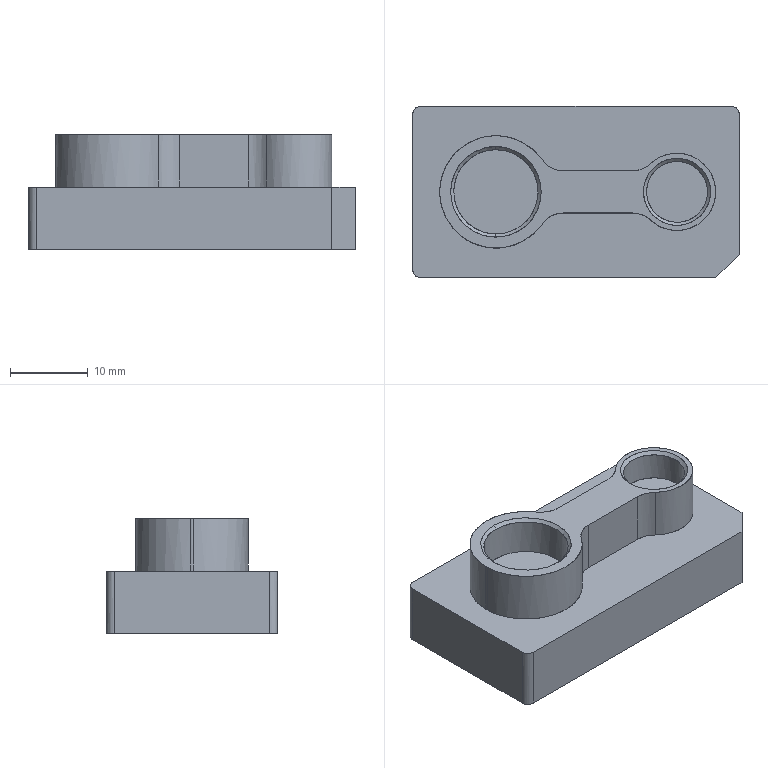NC program | PowerMill | posted by the shop | part box 42 x 22 x 14.721 mm
Lines 3820 to 5389 of 84704:
( TOOL ID   D4C_1_1 )
( TOOL DIA. 4. TIP RAD 0 LENGTH 61.92 )
( Z = -6.85 )
T2 M6
T3
G91 G28 Z0
G0 G90 G54
M08
S18000 M3
X0 Y0 M8
G43 Z9.801 H2
X1.245 Y5.678
Z.792
G1 Z-.408 F3600
X1.235 Y5.658 F6000
G3 X1.324 Y5.393 I.177 J-.089
G1 X2.684 Y4.713
X6.833
X7.571 Y4.749
X7.809 Y4.821
X8.268 Y5.125
X8.864 Y5.613
X9.761 Y6.174
X10.724 Y6.589
X11.713 Y6.85
X12.201 Y6.923
X12.689 Y6.965
X13.177 Y6.97
X13.665 Y6.941
X14.154 Y6.876
X14.642 Y6.777
X15.13 Y6.636
X15.618 Y6.463
X16.369 Y6.101
X17.137 Y5.613
X17.57 Y5.253
X18.058 Y4.796
X18.546 Y4.226
X19.034 Y3.49
X19.209 Y3.172
X19.522 Y2.465
X19.755 Y1.708
X19.861 Y1.22
X19.927 Y.732
X19.96 Y.244
Y-.244
X19.927 Y-.732
X19.861 Y-1.22
X19.755 Y-1.708
X19.522 Y-2.465
X19.209 Y-3.172
X19.034 Y-3.49
X18.604 Y-4.148
X18.058 Y-4.796
X17.714 Y-5.125
X17.137 Y-5.613
X16.369 Y-6.101
X15.618 Y-6.463
X15.282 Y-6.589
X14.642 Y-6.777
X14.154 Y-6.876
X13.665 Y-6.941
X13.177 Y-6.97
X12.689 Y-6.965
X12.201 Y-6.923
X11.713 Y-6.85
X10.737 Y-6.593
X9.761 Y-6.174
X8.864 Y-5.613
X8.268 Y-5.125
X7.809 Y-4.821
X7.571 Y-4.749
X6.833 Y-4.713
X-1.464
X-1.952 Y-4.759
X-2.209 Y-4.849
X-2.329 Y-4.915
X-2.341 Y-4.925
X-2.595 Y-5.125
X-2.609 Y-5.142
X-3.416 Y-6.148
X-3.904 Y-6.654
X-4.392 Y-7.086
X-4.881 Y-7.463
X-5.369 Y-7.799
X-6.345 Y-8.341
X-7.321 Y-8.737
X-8.375 Y-9.029
X-9.273 Y-9.174
X-10.249 Y-9.232
X-11.225 Y-9.186
X-12.201 Y-9.033
X-13.177 Y-8.769
X-13.811 Y-8.541
X-14.642 Y-8.15
X-15.13 Y-7.871
X-15.618 Y-7.547
X-16.232 Y-7.077
X-17.082 Y-6.267
X-17.635 Y-5.613
X-18.288 Y-4.637
X-18.779 Y-3.66
X-19.034 Y-3.005
X-19.267 Y-2.196
X-19.453 Y-1.22
X-19.536 Y-.244
Y.244
X-19.452 Y1.22
X-19.372 Y1.708
X-19.134 Y2.684
X-18.78 Y3.66
X-18.288 Y4.637
X-17.635 Y5.613
X-17.232 Y6.101
X-16.77 Y6.589
X-16.106 Y7.174
X-15.592 Y7.565
X-14.819 Y8.053
X-14.154 Y8.388
X-13.177 Y8.774
X-12.234 Y9.029
X-11.713 Y9.124
X-11.225 Y9.184
X-10.249 Y9.245
X-9.273 Y9.173
X-8.297 Y9.011
X-7.321 Y8.737
X-6.345 Y8.34
X-5.799 Y8.053
X-5.011 Y7.565
X-4.388 Y7.077
X-3.904 Y6.653
X-3.416 Y6.148
X-2.595 Y5.125
X-2.44 Y4.987
X-2.209 Y4.849
X-1.952 Y4.759
X-1.464 Y4.713
X2.684
X1.245 Y5.678 Z-.606
X1.235 Y5.658
G3 X1.324 Y5.393 I.177 J-.089
G1 X2.684 Y4.713
X6.833
X7.571 Y4.749
X7.809 Y4.821
X8.268 Y5.125
X8.864 Y5.613
X9.761 Y6.174
X10.724 Y6.589
X11.713 Y6.85
X12.201 Y6.923
X12.689 Y6.965
X13.177 Y6.97
X13.665 Y6.941
X14.154 Y6.876
X14.642 Y6.777
X15.13 Y6.636
X15.618 Y6.463
X16.369 Y6.101
X17.137 Y5.613
X17.57 Y5.253
X18.058 Y4.796
X18.546 Y4.226
X19.034 Y3.49
X19.209 Y3.172
X19.522 Y2.465
X19.755 Y1.708
X19.861 Y1.22
X19.927 Y.732
X19.96 Y.244
Y-.244
X19.927 Y-.732
X19.861 Y-1.22
X19.755 Y-1.708
X19.522 Y-2.465
X19.209 Y-3.172
X19.034 Y-3.49
X18.604 Y-4.148
X18.058 Y-4.796
X17.714 Y-5.125
X17.137 Y-5.613
X16.369 Y-6.101
X15.618 Y-6.463
X15.282 Y-6.589
X14.642 Y-6.777
X14.154 Y-6.876
X13.665 Y-6.941
X13.177 Y-6.97
X12.689 Y-6.965
X12.201 Y-6.923
X11.713 Y-6.85
X10.737 Y-6.593
X9.761 Y-6.174
X8.864 Y-5.613
X8.268 Y-5.125
X7.809 Y-4.821
X7.571 Y-4.749
X6.833 Y-4.713
X-1.464
X-1.952 Y-4.759
X-2.209 Y-4.849
X-2.329 Y-4.915
X-2.341 Y-4.925
X-2.595 Y-5.125
X-2.609 Y-5.142
X-3.416 Y-6.148
X-3.904 Y-6.654
X-4.392 Y-7.086
X-4.881 Y-7.463
X-5.369 Y-7.799
X-6.345 Y-8.341
X-7.321 Y-8.737
X-8.375 Y-9.029
X-9.273 Y-9.174
X-10.249 Y-9.232
X-11.225 Y-9.186
X-12.201 Y-9.033
X-13.177 Y-8.769
X-13.811 Y-8.541
X-14.642 Y-8.15
X-15.13 Y-7.871
X-15.618 Y-7.547
X-16.232 Y-7.077
X-17.082 Y-6.267
X-17.635 Y-5.613
X-18.288 Y-4.637
X-18.779 Y-3.66
X-19.034 Y-3.005
X-19.267 Y-2.196
X-19.453 Y-1.22
X-19.536 Y-.244
Y.244
X-19.452 Y1.22
X-19.372 Y1.708
X-19.134 Y2.684
X-18.78 Y3.66
X-18.288 Y4.637
X-17.635 Y5.613
X-17.232 Y6.101
X-16.77 Y6.589
X-16.106 Y7.174
X-15.592 Y7.565
X-14.819 Y8.053
X-14.154 Y8.388
X-13.177 Y8.774
X-12.234 Y9.029
X-11.713 Y9.124
X-11.225 Y9.184
X-10.249 Y9.245
X-9.273 Y9.173
X-8.297 Y9.011
X-7.321 Y8.737
X-6.345 Y8.34
X-5.799 Y8.053
X-5.011 Y7.565
X-4.388 Y7.077
X-3.904 Y6.653
X-3.416 Y6.148
X-2.595 Y5.125
X-2.44 Y4.987
X-2.209 Y4.849
X-1.952 Y4.759
X-1.464 Y4.713
X2.684
X1.245 Y5.678 Z-.805
X1.235 Y5.658
G3 X1.324 Y5.393 I.177 J-.089
G1 X2.684 Y4.713
X6.833
X7.571 Y4.749
X7.809 Y4.821
X8.268 Y5.125
X8.864 Y5.613
X9.761 Y6.174
X10.724 Y6.589
X11.713 Y6.85
X12.201 Y6.923
X12.689 Y6.965
X13.177 Y6.97
X13.665 Y6.941
X14.154 Y6.876
X14.642 Y6.777
X15.13 Y6.636
X15.618 Y6.463
X16.369 Y6.101
X17.137 Y5.613
X17.57 Y5.253
X18.058 Y4.796
X18.546 Y4.226
X19.034 Y3.49
X19.209 Y3.172
X19.522 Y2.465
X19.755 Y1.708
X19.861 Y1.22
X19.927 Y.732
X19.96 Y.244
Y-.244
X19.927 Y-.732
X19.861 Y-1.22
X19.755 Y-1.708
X19.522 Y-2.465
X19.209 Y-3.172
X19.034 Y-3.49
X18.604 Y-4.148
X18.058 Y-4.796
X17.714 Y-5.125
X17.137 Y-5.613
X16.369 Y-6.101
X15.618 Y-6.463
X15.282 Y-6.589
X14.642 Y-6.777
X14.154 Y-6.876
X13.665 Y-6.941
X13.177 Y-6.97
X12.689 Y-6.965
X12.201 Y-6.923
X11.713 Y-6.85
X10.737 Y-6.593
X9.761 Y-6.174
X8.864 Y-5.613
X8.268 Y-5.125
X7.809 Y-4.821
X7.571 Y-4.749
X6.833 Y-4.713
X-1.464
X-1.952 Y-4.759
X-2.209 Y-4.849
X-2.329 Y-4.915
X-2.341 Y-4.925
X-2.595 Y-5.125
X-2.609 Y-5.142
X-3.416 Y-6.148
X-3.904 Y-6.654
X-4.392 Y-7.086
X-4.881 Y-7.463
X-5.369 Y-7.799
X-6.345 Y-8.341
X-7.321 Y-8.737
X-8.375 Y-9.029
X-9.273 Y-9.174
X-10.249 Y-9.232
X-11.225 Y-9.186
X-12.201 Y-9.033
X-13.177 Y-8.769
X-13.811 Y-8.541
X-14.642 Y-8.15
X-15.13 Y-7.871
X-15.618 Y-7.547
X-16.232 Y-7.077
X-17.082 Y-6.267
X-17.635 Y-5.613
X-18.288 Y-4.637
X-18.779 Y-3.66
X-19.034 Y-3.005
X-19.267 Y-2.196
X-19.453 Y-1.22
X-19.536 Y-.244
Y.244
X-19.452 Y1.22
X-19.372 Y1.708
X-19.134 Y2.684
X-18.78 Y3.66
X-18.288 Y4.637
X-17.635 Y5.613
X-17.232 Y6.101
X-16.77 Y6.589
X-16.106 Y7.174
X-15.592 Y7.565
X-14.819 Y8.053
X-14.154 Y8.388
X-13.177 Y8.774
X-12.234 Y9.029
X-11.713 Y9.124
X-11.225 Y9.184
X-10.249 Y9.245
X-9.273 Y9.173
X-8.297 Y9.011
X-7.321 Y8.737
X-6.345 Y8.34
X-5.799 Y8.053
X-5.011 Y7.565
X-4.388 Y7.077
X-3.904 Y6.653
X-3.416 Y6.148
X-2.595 Y5.125
X-2.44 Y4.987
X-2.209 Y4.849
X-1.952 Y4.759
X-1.464 Y4.713
X2.684
X1.245 Y5.678 Z-1.004
X1.235 Y5.658
G3 X1.324 Y5.393 I.177 J-.089
G1 X2.684 Y4.713
X6.833
X7.571 Y4.749
X7.809 Y4.821
X8.268 Y5.125
X8.864 Y5.613
X9.761 Y6.174
X10.724 Y6.589
X11.713 Y6.85
X12.201 Y6.923
X12.689 Y6.965
X13.177 Y6.97
X13.665 Y6.941
X14.154 Y6.876
X14.642 Y6.777
X15.13 Y6.636
X15.618 Y6.463
X16.369 Y6.101
X17.137 Y5.613
X17.57 Y5.253
X18.058 Y4.796
X18.546 Y4.226
X19.034 Y3.49
X19.209 Y3.172
X19.522 Y2.465
X19.755 Y1.708
X19.861 Y1.22
X19.927 Y.732
X19.96 Y.244
Y-.244
X19.927 Y-.732
X19.861 Y-1.22
X19.755 Y-1.708
X19.522 Y-2.465
X19.209 Y-3.172
X19.034 Y-3.49
X18.604 Y-4.148
X18.058 Y-4.796
X17.714 Y-5.125
X17.137 Y-5.613
X16.369 Y-6.101
X15.618 Y-6.463
X15.282 Y-6.589
X14.642 Y-6.777
X14.154 Y-6.876
X13.665 Y-6.941
X13.177 Y-6.97
X12.689 Y-6.965
X12.201 Y-6.923
X11.713 Y-6.85
X10.737 Y-6.593
X9.761 Y-6.174
X8.864 Y-5.613
X8.268 Y-5.125
X7.809 Y-4.821
X7.571 Y-4.749
X6.833 Y-4.713
X-1.464
X-1.952 Y-4.759
X-2.209 Y-4.849
X-2.329 Y-4.915
X-2.341 Y-4.925
X-2.595 Y-5.125
X-2.609 Y-5.142
X-3.416 Y-6.148
X-3.904 Y-6.654
X-4.392 Y-7.086
X-4.881 Y-7.463
X-5.369 Y-7.799
X-6.345 Y-8.341
X-7.321 Y-8.737
X-8.375 Y-9.029
X-9.273 Y-9.174
X-10.249 Y-9.232
X-11.225 Y-9.186
X-12.201 Y-9.033
X-13.177 Y-8.769
X-13.811 Y-8.541
X-14.642 Y-8.15
X-15.13 Y-7.871
X-15.618 Y-7.547
X-16.232 Y-7.077
X-17.082 Y-6.267
X-17.635 Y-5.613
X-18.288 Y-4.637
X-18.779 Y-3.66
X-19.034 Y-3.005
X-19.267 Y-2.196
X-19.453 Y-1.22
X-19.536 Y-.244
Y.244
X-19.452 Y1.22
X-19.372 Y1.708
X-19.134 Y2.684
X-18.78 Y3.66
X-18.288 Y4.637
X-17.635 Y5.613
X-17.232 Y6.101
X-16.77 Y6.589
X-16.106 Y7.174
X-15.592 Y7.565
X-14.819 Y8.053
X-14.154 Y8.388
X-13.177 Y8.774
X-12.234 Y9.029
X-11.713 Y9.124
X-11.225 Y9.184
X-10.249 Y9.245
X-9.273 Y9.173
X-8.297 Y9.011
X-7.321 Y8.737
X-6.345 Y8.34
X-5.799 Y8.053
X-5.011 Y7.565
X-4.388 Y7.077
X-3.904 Y6.653
X-3.416 Y6.148
X-2.595 Y5.125
X-2.44 Y4.987
X-2.209 Y4.849
X-1.952 Y4.759
X-1.464 Y4.713
X2.684
X1.245 Y5.678 Z-1.202
X1.235 Y5.658
G3 X1.324 Y5.393 I.177 J-.089
G1 X2.684 Y4.713
X6.833
X7.571 Y4.749
X7.809 Y4.821
X8.268 Y5.125
X8.864 Y5.613
X9.761 Y6.174
X10.724 Y6.589
X11.713 Y6.85
X12.201 Y6.923
X12.689 Y6.965
X13.177 Y6.97
X13.665 Y6.941
X14.154 Y6.876
X14.642 Y6.777
X15.13 Y6.636
X15.618 Y6.463
X16.369 Y6.101
X17.137 Y5.613
X17.57 Y5.253
X18.058 Y4.796
X18.546 Y4.226
X19.034 Y3.49
X19.209 Y3.172
X19.522 Y2.465
X19.755 Y1.708
X19.861 Y1.22
X19.927 Y.732
X19.96 Y.244
Y-.244
X19.927 Y-.732
X19.861 Y-1.22
X19.755 Y-1.708
X19.522 Y-2.465
X19.209 Y-3.172
X19.034 Y-3.49
X18.604 Y-4.148
X18.058 Y-4.796
X17.714 Y-5.125
X17.137 Y-5.613
X16.369 Y-6.101
X15.618 Y-6.463
X15.282 Y-6.589
X14.642 Y-6.777
X14.154 Y-6.876
X13.665 Y-6.941
X13.177 Y-6.97
X12.689 Y-6.965
X12.201 Y-6.923
X11.713 Y-6.85
X10.737 Y-6.593
X9.761 Y-6.174
X8.864 Y-5.613
X8.268 Y-5.125
X7.809 Y-4.821
X7.571 Y-4.749
X6.833 Y-4.713
X-1.464
X-1.952 Y-4.759
X-2.209 Y-4.849
X-2.329 Y-4.915
X-2.341 Y-4.925
X-2.595 Y-5.125
X-2.609 Y-5.142
X-3.416 Y-6.148
X-3.904 Y-6.654
X-4.392 Y-7.086
X-4.881 Y-7.463
X-5.369 Y-7.799
X-6.345 Y-8.341
X-7.321 Y-8.737
X-8.375 Y-9.029
X-9.273 Y-9.174
X-10.249 Y-9.232
X-11.225 Y-9.186
X-12.201 Y-9.033
X-13.177 Y-8.769
X-13.811 Y-8.541
X-14.642 Y-8.15
X-15.13 Y-7.871
X-15.618 Y-7.547
X-16.232 Y-7.077
X-17.082 Y-6.267
X-17.635 Y-5.613
X-18.288 Y-4.637
X-18.779 Y-3.66
X-19.034 Y-3.005
X-19.267 Y-2.196
X-19.453 Y-1.22
X-19.536 Y-.244
Y.244
X-19.452 Y1.22
X-19.372 Y1.708
X-19.134 Y2.684
X-18.78 Y3.66
X-18.288 Y4.637
X-17.635 Y5.613
X-17.232 Y6.101
X-16.77 Y6.589
X-16.106 Y7.174
X-15.592 Y7.565
X-14.819 Y8.053
X-14.154 Y8.388
X-13.177 Y8.774
X-12.234 Y9.029
X-11.713 Y9.124
X-11.225 Y9.184
X-10.249 Y9.245
X-9.273 Y9.173
X-8.297 Y9.011
X-7.321 Y8.737
X-6.345 Y8.34
X-5.799 Y8.053
X-5.011 Y7.565
X-4.388 Y7.077
X-3.904 Y6.653
X-3.416 Y6.148
X-2.595 Y5.125
X-2.44 Y4.987
X-2.209 Y4.849
X-1.952 Y4.759
X-1.464 Y4.713
X2.684
X1.245 Y5.678 Z-1.401
X1.235 Y5.658
G3 X1.324 Y5.393 I.177 J-.089
G1 X2.684 Y4.713
X6.833
X7.571 Y4.749
X7.809 Y4.821
X8.268 Y5.125
X8.864 Y5.613
X9.761 Y6.174
X10.724 Y6.589
X11.713 Y6.85
X12.201 Y6.923
X12.689 Y6.965
X13.177 Y6.97
X13.665 Y6.941
X14.154 Y6.876
X14.642 Y6.777
X15.13 Y6.636
X15.618 Y6.463
X16.369 Y6.101
X17.137 Y5.613
X17.57 Y5.253
X18.058 Y4.796
X18.546 Y4.226
X19.034 Y3.49
X19.209 Y3.172
X19.522 Y2.465
X19.755 Y1.708
X19.861 Y1.22
X19.927 Y.732
X19.96 Y.244
Y-.244
X19.927 Y-.732
X19.861 Y-1.22
X19.755 Y-1.708
X19.522 Y-2.465
X19.209 Y-3.172
X19.034 Y-3.49
X18.604 Y-4.148
X18.058 Y-4.796
X17.714 Y-5.125
X17.137 Y-5.613
X16.369 Y-6.101
X15.618 Y-6.463
X15.282 Y-6.589
X14.642 Y-6.777
X14.154 Y-6.876
X13.665 Y-6.941
X13.177 Y-6.97
X12.689 Y-6.965
X12.201 Y-6.923
X11.713 Y-6.85
X10.737 Y-6.593
X9.761 Y-6.174
X8.864 Y-5.613
X8.268 Y-5.125
X7.809 Y-4.821
X7.571 Y-4.749
X6.833 Y-4.713
X-1.464
X-1.952 Y-4.759
X-2.209 Y-4.849
X-2.329 Y-4.915
X-2.341 Y-4.925
X-2.595 Y-5.125
X-2.609 Y-5.142
X-3.416 Y-6.148
X-3.904 Y-6.654
X-4.392 Y-7.086
X-4.881 Y-7.463
X-5.369 Y-7.799
X-6.345 Y-8.341
X-7.321 Y-8.737
X-8.375 Y-9.029
X-9.273 Y-9.174
X-10.249 Y-9.232
X-11.225 Y-9.186
X-12.201 Y-9.033
X-13.177 Y-8.769
X-13.811 Y-8.541
X-14.642 Y-8.15
X-15.13 Y-7.871
X-15.618 Y-7.547
X-16.232 Y-7.077
X-17.082 Y-6.267
X-17.635 Y-5.613
X-18.288 Y-4.637
X-18.779 Y-3.66
X-19.034 Y-3.005
X-19.267 Y-2.196
X-19.453 Y-1.22
X-19.536 Y-.244
Y.244
X-19.452 Y1.22
X-19.372 Y1.708
X-19.134 Y2.684
X-18.78 Y3.66
X-18.288 Y4.637
X-17.635 Y5.613
X-17.232 Y6.101
X-16.77 Y6.589
X-16.106 Y7.174
X-15.592 Y7.565
X-14.819 Y8.053
X-14.154 Y8.388
X-13.177 Y8.774
X-12.234 Y9.029
X-11.713 Y9.124
X-11.225 Y9.184
X-10.249 Y9.245
X-9.273 Y9.173
X-8.297 Y9.011
X-7.321 Y8.737
X-6.345 Y8.34
X-5.799 Y8.053
X-5.011 Y7.565
X-4.388 Y7.077
X-3.904 Y6.653
X-3.416 Y6.148
X-2.595 Y5.125
X-2.44 Y4.987
X-2.209 Y4.849
X-1.952 Y4.759
X-1.464 Y4.713
X2.684
X1.245 Y5.678 Z-1.6
X1.235 Y5.658
G3 X1.324 Y5.393 I.177 J-.089
G1 X2.684 Y4.713
X6.833
X7.571 Y4.749
X7.809 Y4.821
X8.268 Y5.125
X8.864 Y5.613
X9.761 Y6.174
X10.724 Y6.589
X11.713 Y6.85
X12.201 Y6.923
X12.689 Y6.965
X13.177 Y6.97
X13.665 Y6.941
X14.154 Y6.876
X14.642 Y6.777
X15.13 Y6.636
X15.618 Y6.463
X16.369 Y6.101
X17.137 Y5.613
X17.57 Y5.253
X18.058 Y4.796
X18.546 Y4.226
X19.034 Y3.49
X19.209 Y3.172
X19.522 Y2.465
X19.755 Y1.708
X19.861 Y1.22
X19.927 Y.732
X19.96 Y.244
Y-.244
X19.927 Y-.732
X19.861 Y-1.22
X19.755 Y-1.708
X19.522 Y-2.465
X19.209 Y-3.172
X19.034 Y-3.49
X18.604 Y-4.148
X18.058 Y-4.796
X17.714 Y-5.125
X17.137 Y-5.613
X16.369 Y-6.101
X15.618 Y-6.463
X15.282 Y-6.589
X14.642 Y-6.777
X14.154 Y-6.876
X13.665 Y-6.941
X13.177 Y-6.97
X12.689 Y-6.965
X12.201 Y-6.923
X11.713 Y-6.85
X10.737 Y-6.593
X9.761 Y-6.174
X8.864 Y-5.613
X8.268 Y-5.125
X7.809 Y-4.821
X7.571 Y-4.749
X6.833 Y-4.713
X-1.464
X-1.952 Y-4.759
X-2.209 Y-4.849
X-2.329 Y-4.915
X-2.341 Y-4.925
X-2.595 Y-5.125
X-2.609 Y-5.142
X-3.416 Y-6.148
X-3.904 Y-6.654
X-4.392 Y-7.086
X-4.881 Y-7.463
X-5.369 Y-7.799
X-6.345 Y-8.341
X-7.321 Y-8.737
X-8.375 Y-9.029
X-9.273 Y-9.174
X-10.249 Y-9.232
X-11.225 Y-9.186
X-12.201 Y-9.033
X-13.177 Y-8.769
X-13.811 Y-8.541
X-14.642 Y-8.15
X-15.13 Y-7.871
X-15.618 Y-7.547
X-16.232 Y-7.077
X-17.082 Y-6.267
X-17.635 Y-5.613
X-18.288 Y-4.637
X-18.779 Y-3.66
X-19.034 Y-3.005
X-19.267 Y-2.196
X-19.453 Y-1.22
X-19.536 Y-.244
Y.244
X-19.452 Y1.22
X-19.372 Y1.708
X-19.134 Y2.684
X-18.78 Y3.66
X-18.288 Y4.637
X-17.635 Y5.613
X-17.232 Y6.101
X-16.77 Y6.589
X-16.106 Y7.174
X-15.592 Y7.565
X-14.819 Y8.053
X-14.154 Y8.388
X-13.177 Y8.774
X-12.234 Y9.029
X-11.713 Y9.124
X-11.225 Y9.184
X-10.249 Y9.245
X-9.273 Y9.173
X-8.297 Y9.011
X-7.321 Y8.737
X-6.345 Y8.34
X-5.799 Y8.053
X-5.011 Y7.565
X-4.388 Y7.077
X-3.904 Y6.653
X-3.416 Y6.148
X-2.595 Y5.125
X-2.44 Y4.987
X-2.209 Y4.849
X-1.952 Y4.759
X-1.464 Y4.713
X2.684
X1.245 Y5.678 Z-1.798
X1.235 Y5.658
G3 X1.324 Y5.393 I.177 J-.089
G1 X2.684 Y4.713
X6.833
X7.571 Y4.749
X7.809 Y4.821
X8.268 Y5.125
X8.864 Y5.613
X9.761 Y6.174
X10.724 Y6.589
X11.713 Y6.85
X12.201 Y6.923
X12.689 Y6.965
X13.177 Y6.97
X13.665 Y6.941
X14.154 Y6.876
X14.642 Y6.777
X15.13 Y6.636
X15.618 Y6.463
X16.369 Y6.101
X17.137 Y5.613
X17.57 Y5.253
X18.058 Y4.796
X18.546 Y4.226
X19.034 Y3.49
X19.209 Y3.172
X19.522 Y2.465
X19.755 Y1.708
X19.861 Y1.22
X19.927 Y.732
X19.96 Y.244
Y-.244
X19.927 Y-.732
X19.861 Y-1.22
X19.755 Y-1.708
X19.522 Y-2.465
X19.209 Y-3.172
X19.034 Y-3.49
X18.604 Y-4.148
X18.058 Y-4.796
X17.714 Y-5.125
X17.137 Y-5.613
X16.369 Y-6.101
X15.618 Y-6.463
X15.282 Y-6.589
X14.642 Y-6.777
X14.154 Y-6.876
X13.665 Y-6.941
X13.177 Y-6.97
X12.689 Y-6.965
X12.201 Y-6.923
X11.713 Y-6.85
X10.737 Y-6.593
X9.761 Y-6.174
X8.864 Y-5.613
X8.268 Y-5.125
X7.809 Y-4.821
X7.571 Y-4.749
X6.833 Y-4.713
X-1.464
X-1.952 Y-4.759
X-2.209 Y-4.849
X-2.329 Y-4.915
X-2.341 Y-4.925
X-2.595 Y-5.125
X-2.609 Y-5.142
X-3.416 Y-6.148
X-3.904 Y-6.654
X-4.392 Y-7.086
X-4.881 Y-7.463
X-5.369 Y-7.799
X-6.345 Y-8.341
X-7.321 Y-8.737
X-8.375 Y-9.029
X-9.273 Y-9.174
X-10.249 Y-9.232
X-11.225 Y-9.186
X-12.201 Y-9.033
X-13.177 Y-8.769
X-13.811 Y-8.541
X-14.642 Y-8.15
X-15.13 Y-7.871
X-15.618 Y-7.547
X-16.232 Y-7.077
X-17.082 Y-6.267
X-17.635 Y-5.613
X-18.288 Y-4.637
X-18.779 Y-3.66
X-19.034 Y-3.005
X-19.267 Y-2.196
X-19.453 Y-1.22
X-19.536 Y-.244
Y.244
X-19.452 Y1.22
X-19.372 Y1.708
X-19.134 Y2.684
X-18.78 Y3.66
X-18.288 Y4.637
X-17.635 Y5.613
X-17.232 Y6.101
X-16.77 Y6.589
X-16.106 Y7.174
X-15.592 Y7.565
X-14.819 Y8.053
X-14.154 Y8.388
X-13.177 Y8.774
X-12.234 Y9.029
X-11.713 Y9.124
X-11.225 Y9.184
X-10.249 Y9.245
X-9.273 Y9.173
X-8.297 Y9.011
X-7.321 Y8.737
X-6.345 Y8.34
X-5.799 Y8.053
X-5.011 Y7.565
X-4.388 Y7.077
X-3.904 Y6.653
X-3.416 Y6.148
X-2.595 Y5.125
X-2.44 Y4.987
X-2.209 Y4.849
X-1.952 Y4.759
X-1.464 Y4.713
X2.684
X1.245 Y5.678 Z-1.997
X1.235 Y5.658
G3 X1.324 Y5.393 I.177 J-.089
G1 X2.684 Y4.713
X6.833
X7.571 Y4.749
X7.809 Y4.821
X8.268 Y5.125
X8.864 Y5.613
X9.761 Y6.174
X10.724 Y6.589
X11.713 Y6.85
X12.201 Y6.923
X12.689 Y6.965
X13.177 Y6.97
X13.665 Y6.941
X14.154 Y6.876
X14.642 Y6.777
X15.13 Y6.636
X15.618 Y6.463
X16.369 Y6.101
X17.137 Y5.613
X17.57 Y5.253
X18.058 Y4.796
X18.546 Y4.226
X19.034 Y3.49
X19.209 Y3.172
X19.522 Y2.465
X19.755 Y1.708
X19.861 Y1.22
X19.927 Y.732
X19.96 Y.244
Y-.244
X19.927 Y-.732
X19.861 Y-1.22
X19.755 Y-1.708
X19.522 Y-2.465
X19.209 Y-3.172
X19.034 Y-3.49
X18.604 Y-4.148
X18.058 Y-4.796
X17.714 Y-5.125
X17.137 Y-5.613
X16.369 Y-6.101
X15.618 Y-6.463
X15.282 Y-6.589
X14.642 Y-6.777
X14.154 Y-6.876
X13.665 Y-6.941
X13.177 Y-6.97
X12.689 Y-6.965
X12.201 Y-6.923
X11.713 Y-6.85
X10.737 Y-6.593
X9.761 Y-6.174
X8.864 Y-5.613
X8.268 Y-5.125
X7.809 Y-4.821
X7.571 Y-4.749
X6.833 Y-4.713
X-1.464
X-1.952 Y-4.759
X-2.209 Y-4.849
X-2.329 Y-4.915
X-2.341 Y-4.925
X-2.595 Y-5.125
X-2.609 Y-5.142
X-3.416 Y-6.148
X-3.904 Y-6.654
X-4.392 Y-7.086
X-4.881 Y-7.463
X-5.369 Y-7.799
X-6.345 Y-8.341
X-7.321 Y-8.737
X-8.375 Y-9.029
X-9.273 Y-9.174
X-10.249 Y-9.232
X-11.225 Y-9.186
X-12.201 Y-9.033
X-13.177 Y-8.769
X-13.811 Y-8.541
X-14.642 Y-8.15
X-15.13 Y-7.871
X-15.618 Y-7.547
X-16.232 Y-7.077
X-17.082 Y-6.267
X-17.635 Y-5.613
X-18.288 Y-4.637
X-18.779 Y-3.66
X-19.034 Y-3.005
X-19.267 Y-2.196
X-19.453 Y-1.22
X-19.536 Y-.244
Y.244
X-19.452 Y1.22
X-19.372 Y1.708
X-19.134 Y2.684
X-18.78 Y3.66
X-18.288 Y4.637
X-17.635 Y5.613
X-17.232 Y6.101
X-16.77 Y6.589
X-16.106 Y7.174
X-15.592 Y7.565
X-14.819 Y8.053
X-14.154 Y8.388
X-13.177 Y8.774
X-12.234 Y9.029
X-11.713 Y9.124
X-11.225 Y9.184
X-10.249 Y9.245
X-9.273 Y9.173
X-8.297 Y9.011
X-7.321 Y8.737
X-6.345 Y8.34
X-5.799 Y8.053
X-5.011 Y7.565
X-4.388 Y7.077
X-3.904 Y6.653
X-3.416 Y6.148
X-2.595 Y5.125
X-2.44 Y4.987
X-2.209 Y4.849
X-1.952 Y4.759
X-1.464 Y4.713
X2.684
X1.245 Y5.678 Z-2.196
X1.235 Y5.658
G3 X1.324 Y5.393 I.177 J-.089
G1 X2.684 Y4.713
X6.833
X7.571 Y4.749
X7.809 Y4.821
X8.268 Y5.125
X8.864 Y5.613
X9.761 Y6.174
X10.724 Y6.589
X11.713 Y6.85
X12.201 Y6.923
X12.689 Y6.965
X13.177 Y6.97
X13.665 Y6.941
X14.154 Y6.876
X14.642 Y6.777
X15.13 Y6.636
X15.618 Y6.463
X16.369 Y6.101
X17.137 Y5.613
X17.57 Y5.253
X18.058 Y4.796
X18.546 Y4.226
X19.034 Y3.49
X19.209 Y3.172
X19.522 Y2.465
X19.755 Y1.708
X19.861 Y1.22
X19.927 Y.732
X19.96 Y.244
Y-.244
X19.927 Y-.732
X19.861 Y-1.22
X19.755 Y-1.708
X19.522 Y-2.465
X19.209 Y-3.172
X19.034 Y-3.49
X18.604 Y-4.148
X18.058 Y-4.796
X17.714 Y-5.125
X17.137 Y-5.613
X16.369 Y-6.101
X15.618 Y-6.463
X15.282 Y-6.589
X14.642 Y-6.777
X14.154 Y-6.876
X13.665 Y-6.941
X13.177 Y-6.97
X12.689 Y-6.965
X12.201 Y-6.923
X11.713 Y-6.85
X10.737 Y-6.593
X9.761 Y-6.174
X8.864 Y-5.613
X8.268 Y-5.125
X7.809 Y-4.821
X7.571 Y-4.749
X6.833 Y-4.713
X-1.464
X-1.952 Y-4.759
X-2.209 Y-4.849
X-2.329 Y-4.915
X-2.341 Y-4.925
X-2.595 Y-5.125
X-2.609 Y-5.142
X-3.416 Y-6.148
X-3.904 Y-6.654
X-4.392 Y-7.086
X-4.881 Y-7.463
X-5.369 Y-7.799
X-6.345 Y-8.341
X-7.321 Y-8.737
X-8.375 Y-9.029
X-9.273 Y-9.174
X-10.249 Y-9.232
X-11.225 Y-9.186
X-12.201 Y-9.033
X-13.177 Y-8.769
X-13.811 Y-8.541
X-14.642 Y-8.15
X-15.13 Y-7.871
X-15.618 Y-7.547
X-16.232 Y-7.077
X-17.082 Y-6.267
X-17.635 Y-5.613
X-18.288 Y-4.637
X-18.779 Y-3.66
X-19.034 Y-3.005
X-19.267 Y-2.196
X-19.453 Y-1.22
X-19.536 Y-.244
Y.244
X-19.452 Y1.22
X-19.372 Y1.708
X-19.134 Y2.684
X-18.78 Y3.66
X-18.288 Y4.637
X-17.635 Y5.613
X-17.232 Y6.101
X-16.77 Y6.589
X-16.106 Y7.174
X-15.592 Y7.565
X-14.819 Y8.053
X-14.154 Y8.388
X-13.177 Y8.774
X-12.234 Y9.029
X-11.713 Y9.124
X-11.225 Y9.184
X-10.249 Y9.245
X-9.273 Y9.173
X-8.297 Y9.011
X-7.321 Y8.737
X-6.345 Y8.34
X-5.799 Y8.053
X-5.011 Y7.565
X-4.388 Y7.077
X-3.904 Y6.653
X-3.416 Y6.148
X-2.595 Y5.125
X-2.44 Y4.987
X-2.209 Y4.849
X-1.952 Y4.759
X-1.464 Y4.713
X2.684
X1.245 Y5.678 Z-2.394
X1.235 Y5.658
G3 X1.324 Y5.393 I.177 J-.089
G1 X2.684 Y4.713
X6.833
X7.571 Y4.749
X7.809 Y4.821
X8.268 Y5.125
X8.864 Y5.613
X9.761 Y6.174
X10.724 Y6.589
X11.713 Y6.85
X12.201 Y6.923
X12.689 Y6.965
X13.177 Y6.97
X13.665 Y6.941
X14.154 Y6.876
X14.642 Y6.777
X15.13 Y6.636
X15.618 Y6.463
X16.369 Y6.101
X17.137 Y5.613
X17.57 Y5.253
X18.058 Y4.796
X18.546 Y4.226
X19.034 Y3.49
X19.209 Y3.172
X19.522 Y2.465
X19.755 Y1.708
X19.861 Y1.22
X19.927 Y.732
X19.96 Y.244
Y-.244
X19.927 Y-.732
X19.861 Y-1.22
X19.755 Y-1.708
X19.522 Y-2.465
X19.209 Y-3.172
X19.034 Y-3.49
X18.604 Y-4.148
X18.058 Y-4.796
X17.714 Y-5.125
X17.137 Y-5.613
X16.369 Y-6.101
X15.618 Y-6.463
X15.282 Y-6.589
X14.642 Y-6.777
X14.154 Y-6.876
X13.665 Y-6.941
X13.177 Y-6.97
X12.689 Y-6.965
X12.201 Y-6.923
X11.713 Y-6.85
X10.737 Y-6.593
X9.761 Y-6.174
X8.864 Y-5.613
X8.268 Y-5.125
X7.809 Y-4.821
X7.571 Y-4.749
X6.833 Y-4.713
X-1.464
X-1.952 Y-4.759
X-2.209 Y-4.849
X-2.329 Y-4.915
X-2.341 Y-4.925
X-2.595 Y-5.125
X-2.609 Y-5.142
X-3.416 Y-6.148
X-3.904 Y-6.654
X-4.392 Y-7.086
X-4.881 Y-7.463
X-5.369 Y-7.799
X-6.345 Y-8.341
X-7.321 Y-8.737
X-8.375 Y-9.029
X-9.273 Y-9.174
X-10.249 Y-9.232
X-11.225 Y-9.186
X-12.201 Y-9.033
X-13.177 Y-8.769
X-13.811 Y-8.541
X-14.642 Y-8.15
X-15.13 Y-7.871
X-15.618 Y-7.547
X-16.232 Y-7.077
X-17.082 Y-6.267
X-17.635 Y-5.613
X-18.288 Y-4.637
X-18.779 Y-3.66
X-19.034 Y-3.005
X-19.267 Y-2.196
X-19.453 Y-1.22
X-19.536 Y-.244
Y.244
X-19.452 Y1.22
X-19.372 Y1.708
X-19.134 Y2.684
X-18.78 Y3.66
X-18.288 Y4.637
X-17.635 Y5.613
X-17.232 Y6.101
X-16.77 Y6.589
X-16.106 Y7.174
X-15.592 Y7.565
X-14.819 Y8.053
X-14.154 Y8.388
X-13.177 Y8.774
X-12.234 Y9.029
X-11.713 Y9.124
X-11.225 Y9.184
X-10.249 Y9.245
X-9.273 Y9.173
X-8.297 Y9.011
X-7.321 Y8.737
X-6.345 Y8.34
X-5.799 Y8.053
X-5.011 Y7.565
X-4.388 Y7.077
X-3.904 Y6.653
X-3.416 Y6.148
X-2.595 Y5.125
X-2.44 Y4.987
X-2.209 Y4.849
X-1.952 Y4.759
X-1.464 Y4.713
X2.684
X1.245 Y5.678 Z-2.593
X1.235 Y5.658
G3 X1.324 Y5.393 I.177 J-.089
G1 X2.684 Y4.713
X6.833
X7.572 Y4.749
X7.809 Y4.821
X8.268 Y5.125
X8.864 Y5.613
X9.761 Y6.174
X10.724 Y6.589
X11.713 Y6.85
X12.201 Y6.923
X12.689 Y6.965
X13.177 Y6.97
X13.665 Y6.941
X14.154 Y6.876
X14.642 Y6.777
X15.13 Y6.636
X15.618 Y6.463
X16.369 Y6.101
X17.137 Y5.613
X17.57 Y5.253
X18.058 Y4.796
X18.546 Y4.226
X19.034 Y3.49
X19.209 Y3.172
X19.522 Y2.465
X19.755 Y1.708
X19.861 Y1.22
X19.927 Y.732
X19.96 Y.244
Y-.244
X19.927 Y-.732
X19.861 Y-1.22
X19.755 Y-1.708
X19.522 Y-2.465
X19.209 Y-3.172
X19.034 Y-3.49
X18.604 Y-4.148
X18.058 Y-4.796
X17.714 Y-5.125
X17.137 Y-5.613
X16.369 Y-6.101
X15.618 Y-6.463
X15.282 Y-6.589
X14.642 Y-6.777
X14.154 Y-6.876
X13.665 Y-6.941
X13.177 Y-6.97
X12.689 Y-6.965
X12.201 Y-6.923
X11.713 Y-6.85
X10.737 Y-6.593
X9.761 Y-6.174
X8.864 Y-5.613
X8.268 Y-5.125
X7.809 Y-4.821
X7.572 Y-4.749
X6.833 Y-4.713
X-1.464
X-1.952 Y-4.759
X-2.209 Y-4.849
X-2.329 Y-4.915
X-2.341 Y-4.925
X-2.595 Y-5.125
X-2.609 Y-5.142
X-3.416 Y-6.148
X-3.904 Y-6.654
X-4.392 Y-7.086
X-4.881 Y-7.463
X-5.369 Y-7.799
X-6.345 Y-8.341
X-7.321 Y-8.737
X-8.375 Y-9.029
X-9.273 Y-9.174
X-10.249 Y-9.232
X-11.225 Y-9.186
X-12.201 Y-9.033
X-13.177 Y-8.769
X-13.811 Y-8.541
X-14.642 Y-8.15
X-15.13 Y-7.871
X-15.618 Y-7.547
X-16.232 Y-7.077
X-17.082 Y-6.267
X-17.635 Y-5.613
X-18.288 Y-4.637
X-18.779 Y-3.66
X-19.034 Y-3.005
X-19.267 Y-2.196
X-19.453 Y-1.22
X-19.536 Y-.244
Y.244
X-19.452 Y1.22
X-19.372 Y1.708
X-19.134 Y2.684
X-18.78 Y3.66
X-18.288 Y4.637
X-17.635 Y5.613
X-17.232 Y6.101
X-16.77 Y6.589
X-16.106 Y7.174
X-15.592 Y7.565
X-14.819 Y8.053
X-14.154 Y8.388
X-13.177 Y8.774
X-12.234 Y9.029
X-11.713 Y9.124
X-11.225 Y9.184
X-10.249 Y9.245
X-9.273 Y9.173
X-8.297 Y9.011
X-7.321 Y8.737
X-6.345 Y8.34
X-5.799 Y8.053
X-5.011 Y7.565
X-4.388 Y7.077
X-3.904 Y6.653
X-3.416 Y6.148
X-2.595 Y5.125
X-2.44 Y4.987
X-2.209 Y4.849
X-1.952 Y4.759
X-1.464 Y4.713
X2.684
X1.245 Y5.678 Z-2.792
X1.235 Y5.658
G3 X1.324 Y5.393 I.177 J-.089
G1 X2.684 Y4.713
X6.833
X7.572 Y4.749
X7.809 Y4.821
X8.268 Y5.125
X8.864 Y5.613
X9.761 Y6.174
X10.724 Y6.589
X11.713 Y6.85
X12.201 Y6.923
X12.689 Y6.965
X13.177 Y6.97
X13.665 Y6.941
X14.154 Y6.876
X14.642 Y6.777
X15.13 Y6.636
X15.618 Y6.463
X16.369 Y6.101
X17.137 Y5.613
X17.57 Y5.253
X18.058 Y4.796
X18.546 Y4.226
X19.034 Y3.49
X19.209 Y3.172
X19.522 Y2.465
X19.755 Y1.708
X19.861 Y1.22
X19.927 Y.732
X19.96 Y.244
Y-.244
X19.927 Y-.732
X19.861 Y-1.22
X19.755 Y-1.708
X19.522 Y-2.465
X19.209 Y-3.172
X19.034 Y-3.49
X18.604 Y-4.148
X18.058 Y-4.796
X17.714 Y-5.125
X17.137 Y-5.613
X16.369 Y-6.101
X15.618 Y-6.463